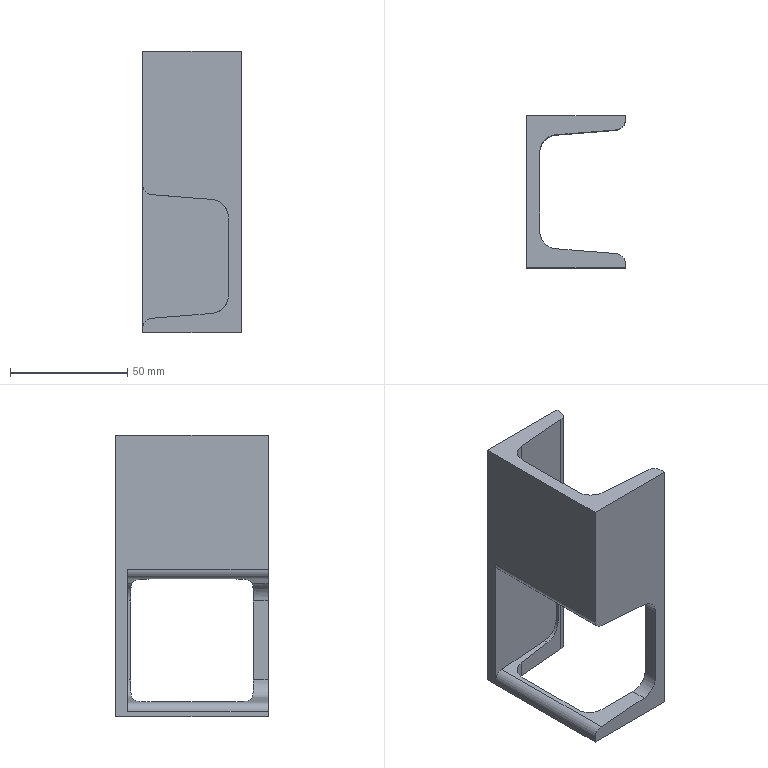Part | STEP file | DIN 1026-1 U 65 1785416005636 | 1 solid | 28 faces | box 42 x 65 x 120 mm | volume 74132 mm3 | plane 16 | cylinder 12 | commonest cylinder face diameters 15 x8 8 x4
STEP:
#1=CARTESIAN_POINT('',(29.598,-25.688,56.812));
#2=VERTEX_POINT('',#1);
#3=CARTESIAN_POINT('',(12.402,-24.312,58.188));
#4=VERTEX_POINT('',#3);
#5=CARTESIAN_POINT('',(10.69,-24.175,58.325));
#6=DIRECTION('',(-0.9937,0.07949,0.07949));
#7=VECTOR('',#6,10.);
#8=LINE('',#5,#7);
#9=EDGE_CURVE('',#2,#4,#8,.T.);
#10=ORIENTED_EDGE('',*,*,#9,.F.);
#11=CARTESIAN_POINT('',(29.598,-32.5,56.812));
#12=VERTEX_POINT('',#11);
#13=CARTESIAN_POINT('',(29.598,-32.5,56.812));
#14=DIRECTION('',(0.,1.,0.));
#15=VECTOR('',#14,10.);
#16=LINE('',#13,#15);
#17=EDGE_CURVE('',#12,#2,#16,.T.);
#18=ORIENTED_EDGE('',*,*,#17,.F.);
#19=CARTESIAN_POINT('',(3.681,-32.5,58.886));
#20=VERTEX_POINT('',#19);
#21=CARTESIAN_POINT('',(25.059,-32.5,57.175));
#22=DIRECTION('',(0.9968,0.,-0.07975));
#23=VECTOR('',#22,10.);
#24=LINE('',#21,#23);
#25=EDGE_CURVE('',#20,#12,#24,.T.);
#26=ORIENTED_EDGE('',*,*,#25,.F.);
#27=CARTESIAN_POINT('',(3.681,27.5,58.886));
#28=VERTEX_POINT('',#27);
#29=CARTESIAN_POINT('',(3.681,-32.5,58.886));
#30=DIRECTION('',(0.,1.,0.));
#31=VECTOR('',#30,10.);
#32=LINE('',#29,#31);
#33=EDGE_CURVE('',#20,#28,#32,.T.);
#34=ORIENTED_EDGE('',*,*,#33,.T.);
#35=CARTESIAN_POINT('',(29.598,27.5,56.812));
#36=VERTEX_POINT('',#35);
#37=CARTESIAN_POINT('',(29.598,27.5,56.812));
#38=DIRECTION('',(0.9968,0.,-0.07975));
#39=VECTOR('',#38,10.);
#40=LINE('',#37,#39);
#41=EDGE_CURVE('',#28,#36,#40,.T.);
#42=ORIENTED_EDGE('',*,*,#41,.T.);
#43=CARTESIAN_POINT('',(29.598,25.688,56.812));
#44=VERTEX_POINT('',#43);
#45=CARTESIAN_POINT('',(29.598,-32.5,56.812));
#46=DIRECTION('',(0.,1.,0.));
#47=VECTOR('',#46,10.);
#48=LINE('',#45,#47);
#49=EDGE_CURVE('',#44,#36,#48,.T.);
#50=ORIENTED_EDGE('',*,*,#49,.F.);
#51=CARTESIAN_POINT('',(12.402,24.312,58.188));
#52=VERTEX_POINT('',#51);
#53=CARTESIAN_POINT('',(21.,25.,57.5));
#54=DIRECTION('',(0.9937,0.07949,-0.07949));
#55=VECTOR('',#54,10.);
#56=LINE('',#53,#55);
#57=EDGE_CURVE('',#52,#44,#56,.T.);
#58=ORIENTED_EDGE('',*,*,#57,.F.);
#59=CARTESIAN_POINT('',(5.5,16.836,58.74));
#60=VERTEX_POINT('',#59);
#61=CARTESIAN_POINT('',(13.,16.836,58.14));
#62=DIRECTION('',(-0.07975,0.,-0.9968));
#63=DIRECTION('',(-0.9968,0.,0.07975));
#64=AXIS2_PLACEMENT_3D('',#61,#62,#63);
#65=ELLIPSE('',#64,7.524,7.5);
#66=EDGE_CURVE('',#60,#52,#65,.T.);
#67=ORIENTED_EDGE('',*,*,#66,.F.);
#68=CARTESIAN_POINT('',(5.5,-16.836,58.74));
#69=VERTEX_POINT('',#68);
#70=CARTESIAN_POINT('',(5.5,-16.25,58.74));
#71=DIRECTION('',(0.,1.,0.));
#72=VECTOR('',#71,10.);
#73=LINE('',#70,#72);
#74=EDGE_CURVE('',#69,#60,#73,.T.);
#75=ORIENTED_EDGE('',*,*,#74,.F.);
#76=CARTESIAN_POINT('',(13.,-16.836,58.14));
#77=DIRECTION('',(-0.07975,0.,-0.9968));
#78=DIRECTION('',(-0.9968,0.,0.07975));
#79=AXIS2_PLACEMENT_3D('',#76,#77,#78);
#80=ELLIPSE('',#79,7.524,7.5);
#81=EDGE_CURVE('',#4,#69,#80,.T.);
#82=ORIENTED_EDGE('',*,*,#81,.F.);
#83=EDGE_LOOP('',(#10,#18,#26,#34,#42,#50,#58,#67,#75,#82));
#84=FACE_OUTER_BOUND('',#83,.T.);
#85=CARTESIAN_POINT('',(3.681,-32.5,58.886));
#86=DIRECTION('',(0.07975,0.,0.9968));
#87=DIRECTION('',(0.9968,0.,-0.07975));
#88=AXIS2_PLACEMENT_3D('',#85,#86,#87);
#89=PLANE('',#88);
#90=ADVANCED_FACE('',(#84),#89,.F.);
#91=CARTESIAN_POINT('',(36.5,26.24,49.336));
#92=VERTEX_POINT('',#91);
#93=CARTESIAN_POINT('',(29.,25.64,49.336));
#94=DIRECTION('',(-0.07975,0.9968,0.));
#95=DIRECTION('',(0.9968,0.07975,0.));
#96=AXIS2_PLACEMENT_3D('',#93,#94,#95);
#97=ELLIPSE('',#96,7.524,7.5);
#98=EDGE_CURVE('',#44,#92,#97,.T.);
#99=ORIENTED_EDGE('',*,*,#98,.F.);
#100=ORIENTED_EDGE('',*,*,#49,.T.);
#101=CARTESIAN_POINT('',(36.5,27.5,49.336));
#102=VERTEX_POINT('',#101);
#103=CARTESIAN_POINT('',(29.,27.5,49.336));
#104=DIRECTION('',(0.,1.,0.));
#105=DIRECTION('',(1.,0.,0.));
#106=AXIS2_PLACEMENT_3D('',#103,#104,#105);
#107=CIRCLE('',#106,7.5);
#108=EDGE_CURVE('',#36,#102,#107,.T.);
#109=ORIENTED_EDGE('',*,*,#108,.T.);
#110=CARTESIAN_POINT('',(36.5,-32.5,49.336));
#111=DIRECTION('',(0.,1.,0.));
#112=VECTOR('',#111,10.);
#113=LINE('',#110,#112);
#114=EDGE_CURVE('',#92,#102,#113,.T.);
#115=ORIENTED_EDGE('',*,*,#114,.F.);
#116=EDGE_LOOP('',(#99,#100,#109,#115));
#117=FACE_OUTER_BOUND('',#116,.T.);
#118=CARTESIAN_POINT('',(29.,-32.5,49.336));
#119=DIRECTION('',(0.,1.,0.));
#120=DIRECTION('',(1.,0.,0.));
#121=AXIS2_PLACEMENT_3D('',#118,#119,#120);
#122=CYLINDRICAL_SURFACE('',#121,7.5);
#123=ADVANCED_FACE('',(#117),#122,.F.);
#124=CARTESIAN_POINT('',(36.5,26.24,15.664));
#125=VERTEX_POINT('',#124);
#126=CARTESIAN_POINT('',(36.5,26.24,24.668));
#127=DIRECTION('',(0.,0.,-1.));
#128=VECTOR('',#127,10.);
#129=LINE('',#126,#128);
#130=EDGE_CURVE('',#92,#125,#129,.T.);
#131=ORIENTED_EDGE('',*,*,#130,.F.);
#132=ORIENTED_EDGE('',*,*,#114,.T.);
#133=CARTESIAN_POINT('',(36.5,27.5,15.664));
#134=VERTEX_POINT('',#133);
#135=CARTESIAN_POINT('',(36.5,27.5,15.664));
#136=DIRECTION('',(0.,0.,-1.));
#137=VECTOR('',#136,10.);
#138=LINE('',#135,#137);
#139=EDGE_CURVE('',#102,#134,#138,.T.);
#140=ORIENTED_EDGE('',*,*,#139,.T.);
#141=CARTESIAN_POINT('',(36.5,-32.5,15.664));
#142=DIRECTION('',(0.,1.,0.));
#143=VECTOR('',#142,10.);
#144=LINE('',#141,#143);
#145=EDGE_CURVE('',#125,#134,#144,.T.);
#146=ORIENTED_EDGE('',*,*,#145,.F.);
#147=EDGE_LOOP('',(#131,#132,#140,#146));
#148=FACE_OUTER_BOUND('',#147,.T.);
#149=CARTESIAN_POINT('',(36.5,-32.5,49.336));
#150=DIRECTION('',(1.,0.,0.));
#151=DIRECTION('',(0.,0.,-1.));
#152=AXIS2_PLACEMENT_3D('',#149,#150,#151);
#153=PLANE('',#152);
#154=ADVANCED_FACE('',(#148),#153,.F.);
#155=CARTESIAN_POINT('',(29.598,25.688,8.188));
#156=VERTEX_POINT('',#155);
#157=CARTESIAN_POINT('',(29.,25.64,15.664));
#158=DIRECTION('',(-0.07975,0.9968,0.));
#159=DIRECTION('',(0.9968,0.07975,0.));
#160=AXIS2_PLACEMENT_3D('',#157,#158,#159);
#161=ELLIPSE('',#160,7.524,7.5);
#162=EDGE_CURVE('',#125,#156,#161,.T.);
#163=ORIENTED_EDGE('',*,*,#162,.F.);
#164=ORIENTED_EDGE('',*,*,#145,.T.);
#165=CARTESIAN_POINT('',(29.598,27.5,8.188));
#166=VERTEX_POINT('',#165);
#167=CARTESIAN_POINT('',(29.,27.5,15.664));
#168=DIRECTION('',(0.,1.,0.));
#169=DIRECTION('',(0.07975,0.,-0.9968));
#170=AXIS2_PLACEMENT_3D('',#167,#168,#169);
#171=CIRCLE('',#170,7.5);
#172=EDGE_CURVE('',#134,#166,#171,.T.);
#173=ORIENTED_EDGE('',*,*,#172,.T.);
#174=CARTESIAN_POINT('',(29.598,-32.5,8.188));
#175=DIRECTION('',(0.,1.,0.));
#176=VECTOR('',#175,10.);
#177=LINE('',#174,#176);
#178=EDGE_CURVE('',#156,#166,#177,.T.);
#179=ORIENTED_EDGE('',*,*,#178,.F.);
#180=EDGE_LOOP('',(#163,#164,#173,#179));
#181=FACE_OUTER_BOUND('',#180,.T.);
#182=CARTESIAN_POINT('',(29.,-32.5,15.664));
#183=DIRECTION('',(0.,1.,0.));
#184=DIRECTION('',(0.07975,0.,-0.9968));
#185=AXIS2_PLACEMENT_3D('',#182,#183,#184);
#186=CYLINDRICAL_SURFACE('',#185,7.5);
#187=ADVANCED_FACE('',(#181),#186,.F.);
#188=CARTESIAN_POINT('',(36.5,-26.24,15.664));
#189=VERTEX_POINT('',#188);
#190=CARTESIAN_POINT('',(36.5,-26.24,49.336));
#191=VERTEX_POINT('',#190);
#192=CARTESIAN_POINT('',(36.5,-26.24,24.668));
#193=DIRECTION('',(0.,0.,1.));
#194=VECTOR('',#193,10.);
#195=LINE('',#192,#194);
#196=EDGE_CURVE('',#189,#191,#195,.T.);
#197=ORIENTED_EDGE('',*,*,#196,.F.);
#198=CARTESIAN_POINT('',(36.5,-32.5,15.664));
#199=VERTEX_POINT('',#198);
#200=CARTESIAN_POINT('',(36.5,-32.5,15.664));
#201=DIRECTION('',(0.,1.,0.));
#202=VECTOR('',#201,10.);
#203=LINE('',#200,#202);
#204=EDGE_CURVE('',#199,#189,#203,.T.);
#205=ORIENTED_EDGE('',*,*,#204,.F.);
#206=CARTESIAN_POINT('',(36.5,-32.5,49.336));
#207=VERTEX_POINT('',#206);
#208=CARTESIAN_POINT('',(36.5,-32.5,24.668));
#209=DIRECTION('',(0.,0.,-1.));
#210=VECTOR('',#209,10.);
#211=LINE('',#208,#210);
#212=EDGE_CURVE('',#207,#199,#211,.T.);
#213=ORIENTED_EDGE('',*,*,#212,.F.);
#214=CARTESIAN_POINT('',(36.5,-32.5,49.336));
#215=DIRECTION('',(0.,1.,0.));
#216=VECTOR('',#215,10.);
#217=LINE('',#214,#216);
#218=EDGE_CURVE('',#207,#191,#217,.T.);
#219=ORIENTED_EDGE('',*,*,#218,.T.);
#220=EDGE_LOOP('',(#197,#205,#213,#219));
#221=FACE_OUTER_BOUND('',#220,.T.);
#222=CARTESIAN_POINT('',(36.5,-32.5,49.336));
#223=DIRECTION('',(1.,0.,0.));
#224=DIRECTION('',(0.,0.,-1.));
#225=AXIS2_PLACEMENT_3D('',#222,#223,#224);
#226=PLANE('',#225);
#227=ADVANCED_FACE('',(#221),#226,.F.);
#228=CARTESIAN_POINT('',(29.,-25.64,49.336));
#229=DIRECTION('',(-0.07975,-0.9968,0.));
#230=DIRECTION('',(0.9968,-0.07975,0.));
#231=AXIS2_PLACEMENT_3D('',#228,#229,#230);
#232=ELLIPSE('',#231,7.524,7.5);
#233=EDGE_CURVE('',#191,#2,#232,.T.);
#234=ORIENTED_EDGE('',*,*,#233,.F.);
#235=ORIENTED_EDGE('',*,*,#218,.F.);
#236=CARTESIAN_POINT('',(29.,-32.5,49.336));
#237=DIRECTION('',(0.,1.,0.));
#238=DIRECTION('',(1.,0.,0.));
#239=AXIS2_PLACEMENT_3D('',#236,#237,#238);
#240=CIRCLE('',#239,7.5);
#241=EDGE_CURVE('',#12,#207,#240,.T.);
#242=ORIENTED_EDGE('',*,*,#241,.F.);
#243=ORIENTED_EDGE('',*,*,#17,.T.);
#244=EDGE_LOOP('',(#234,#235,#242,#243));
#245=FACE_OUTER_BOUND('',#244,.T.);
#246=CARTESIAN_POINT('',(29.,-32.5,49.336));
#247=DIRECTION('',(0.,1.,0.));
#248=DIRECTION('',(1.,0.,0.));
#249=AXIS2_PLACEMENT_3D('',#246,#247,#248);
#250=CYLINDRICAL_SURFACE('',#249,7.5);
#251=ADVANCED_FACE('',(#245),#250,.F.);
#252=CARTESIAN_POINT('',(0.,-32.5,62.873));
#253=VERTEX_POINT('',#252);
#254=CARTESIAN_POINT('',(4.,-32.5,62.873));
#255=DIRECTION('',(0.,-1.,0.));
#256=DIRECTION('',(1.,0.,0.));
#257=AXIS2_PLACEMENT_3D('',#254,#255,#256);
#258=CIRCLE('',#257,4.);
#259=EDGE_CURVE('',#253,#20,#258,.T.);
#260=ORIENTED_EDGE('',*,*,#259,.F.);
#261=CARTESIAN_POINT('',(0.,27.5,62.873));
#262=VERTEX_POINT('',#261);
#263=CARTESIAN_POINT('',(0.,-32.5,62.873));
#264=DIRECTION('',(0.,-1.,0.));
#265=VECTOR('',#264,10.);
#266=LINE('',#263,#265);
#267=EDGE_CURVE('',#262,#253,#266,.T.);
#268=ORIENTED_EDGE('',*,*,#267,.F.);
#269=CARTESIAN_POINT('',(4.,27.5,62.873));
#270=DIRECTION('',(0.,-1.,0.));
#271=DIRECTION('',(1.,0.,0.));
#272=AXIS2_PLACEMENT_3D('',#269,#270,#271);
#273=CIRCLE('',#272,4.);
#274=EDGE_CURVE('',#262,#28,#273,.T.);
#275=ORIENTED_EDGE('',*,*,#274,.T.);
#276=ORIENTED_EDGE('',*,*,#33,.F.);
#277=EDGE_LOOP('',(#260,#268,#275,#276));
#278=FACE_OUTER_BOUND('',#277,.T.);
#279=CARTESIAN_POINT('',(4.,-32.5,62.873));
#280=DIRECTION('',(0.,1.,0.));
#281=DIRECTION('',(1.,0.,0.));
#282=AXIS2_PLACEMENT_3D('',#279,#280,#281);
#283=CYLINDRICAL_SURFACE('',#282,4.);
#284=ADVANCED_FACE('',(#278),#283,.T.);
#285=CARTESIAN_POINT('',(3.681,-32.5,6.114));
#286=VERTEX_POINT('',#285);
#287=CARTESIAN_POINT('',(0.,-32.5,2.127));
#288=VERTEX_POINT('',#287);
#289=CARTESIAN_POINT('',(4.,-32.5,2.127));
#290=DIRECTION('',(0.,-1.,0.));
#291=DIRECTION('',(0.07975,0.,-0.9968));
#292=AXIS2_PLACEMENT_3D('',#289,#290,#291);
#293=CIRCLE('',#292,4.);
#294=EDGE_CURVE('',#286,#288,#293,.T.);
#295=ORIENTED_EDGE('',*,*,#294,.F.);
#296=CARTESIAN_POINT('',(3.681,27.5,6.114));
#297=VERTEX_POINT('',#296);
#298=CARTESIAN_POINT('',(3.681,-32.5,6.114));
#299=DIRECTION('',(0.,1.,0.));
#300=VECTOR('',#299,10.);
#301=LINE('',#298,#300);
#302=EDGE_CURVE('',#286,#297,#301,.T.);
#303=ORIENTED_EDGE('',*,*,#302,.T.);
#304=CARTESIAN_POINT('',(0.,27.5,2.127));
#305=VERTEX_POINT('',#304);
#306=CARTESIAN_POINT('',(4.,27.5,2.127));
#307=DIRECTION('',(0.,-1.,0.));
#308=DIRECTION('',(0.07975,0.,-0.9968));
#309=AXIS2_PLACEMENT_3D('',#306,#307,#308);
#310=CIRCLE('',#309,4.);
#311=EDGE_CURVE('',#297,#305,#310,.T.);
#312=ORIENTED_EDGE('',*,*,#311,.T.);
#313=CARTESIAN_POINT('',(0.,-32.5,2.127));
#314=DIRECTION('',(0.,-1.,0.));
#315=VECTOR('',#314,10.);
#316=LINE('',#313,#315);
#317=EDGE_CURVE('',#305,#288,#316,.T.);
#318=ORIENTED_EDGE('',*,*,#317,.T.);
#319=EDGE_LOOP('',(#295,#303,#312,#318));
#320=FACE_OUTER_BOUND('',#319,.T.);
#321=CARTESIAN_POINT('',(4.,-32.5,2.127));
#322=DIRECTION('',(0.,1.,0.));
#323=DIRECTION('',(0.07975,0.,-0.9968));
#324=AXIS2_PLACEMENT_3D('',#321,#322,#323);
#325=CYLINDRICAL_SURFACE('',#324,4.);
#326=ADVANCED_FACE('',(#320),#325,.T.);
#327=CARTESIAN_POINT('',(12.402,-24.312,6.812));
#328=VERTEX_POINT('',#327);
#329=CARTESIAN_POINT('',(29.598,-25.688,8.188));
#330=VERTEX_POINT('',#329);
#331=CARTESIAN_POINT('',(21.,-25.,7.5));
#332=DIRECTION('',(0.9937,-0.07949,0.07949));
#333=VECTOR('',#332,10.);
#334=LINE('',#331,#333);
#335=EDGE_CURVE('',#328,#330,#334,.T.);
#336=ORIENTED_EDGE('',*,*,#335,.F.);
#337=CARTESIAN_POINT('',(5.5,-16.836,6.26));
#338=VERTEX_POINT('',#337);
#339=CARTESIAN_POINT('',(13.,-16.836,6.86));
#340=DIRECTION('',(-0.07975,0.,0.9968));
#341=DIRECTION('',(-0.9968,0.,-0.07975));
#342=AXIS2_PLACEMENT_3D('',#339,#340,#341);
#343=ELLIPSE('',#342,7.524,7.5);
#344=EDGE_CURVE('',#338,#328,#343,.T.);
#345=ORIENTED_EDGE('',*,*,#344,.F.);
#346=CARTESIAN_POINT('',(5.5,16.836,6.26));
#347=VERTEX_POINT('',#346);
#348=CARTESIAN_POINT('',(5.5,-16.25,6.26));
#349=DIRECTION('',(0.,-1.,0.));
#350=VECTOR('',#349,10.);
#351=LINE('',#348,#350);
#352=EDGE_CURVE('',#347,#338,#351,.T.);
#353=ORIENTED_EDGE('',*,*,#352,.F.);
#354=CARTESIAN_POINT('',(12.402,24.312,6.812));
#355=VERTEX_POINT('',#354);
#356=CARTESIAN_POINT('',(13.,16.836,6.86));
#357=DIRECTION('',(-0.07975,0.,0.9968));
#358=DIRECTION('',(-0.9968,0.,-0.07975));
#359=AXIS2_PLACEMENT_3D('',#356,#357,#358);
#360=ELLIPSE('',#359,7.524,7.5);
#361=EDGE_CURVE('',#355,#347,#360,.T.);
#362=ORIENTED_EDGE('',*,*,#361,.F.);
#363=CARTESIAN_POINT('',(31.31,25.825,8.325));
#364=DIRECTION('',(-0.9937,-0.07949,-0.07949));
#365=VECTOR('',#364,10.);
#366=LINE('',#363,#365);
#367=EDGE_CURVE('',#156,#355,#366,.T.);
#368=ORIENTED_EDGE('',*,*,#367,.F.);
#369=ORIENTED_EDGE('',*,*,#178,.T.);
#370=CARTESIAN_POINT('',(3.681,27.5,6.114));
#371=DIRECTION('',(-0.9968,0.,-0.07975));
#372=VECTOR('',#371,10.);
#373=LINE('',#370,#372);
#374=EDGE_CURVE('',#166,#297,#373,.T.);
#375=ORIENTED_EDGE('',*,*,#374,.T.);
#376=ORIENTED_EDGE('',*,*,#302,.F.);
#377=CARTESIAN_POINT('',(29.598,-32.5,8.188));
#378=VERTEX_POINT('',#377);
#379=CARTESIAN_POINT('',(35.434,-32.5,8.655));
#380=DIRECTION('',(-0.9968,0.,-0.07975));
#381=VECTOR('',#380,10.);
#382=LINE('',#379,#381);
#383=EDGE_CURVE('',#378,#286,#382,.T.);
#384=ORIENTED_EDGE('',*,*,#383,.F.);
#385=CARTESIAN_POINT('',(29.598,-32.5,8.188));
#386=DIRECTION('',(0.,1.,0.));
#387=VECTOR('',#386,10.);
#388=LINE('',#385,#387);
#389=EDGE_CURVE('',#378,#330,#388,.T.);
#390=ORIENTED_EDGE('',*,*,#389,.T.);
#391=EDGE_LOOP('',(#336,#345,#353,#362,#368,#369,#375,#376,#384,#390));
#392=FACE_OUTER_BOUND('',#391,.T.);
#393=CARTESIAN_POINT('',(29.598,-32.5,8.188));
#394=DIRECTION('',(0.07975,0.,-0.9968));
#395=DIRECTION('',(-0.9968,0.,-0.07975));
#396=AXIS2_PLACEMENT_3D('',#393,#394,#395);
#397=PLANE('',#396);
#398=ADVANCED_FACE('',(#392),#397,.F.);
#399=CARTESIAN_POINT('',(29.,-25.64,15.664));
#400=DIRECTION('',(-0.07975,-0.9968,0.));
#401=DIRECTION('',(0.9968,-0.07975,0.));
#402=AXIS2_PLACEMENT_3D('',#399,#400,#401);
#403=ELLIPSE('',#402,7.524,7.5);
#404=EDGE_CURVE('',#330,#189,#403,.T.);
#405=ORIENTED_EDGE('',*,*,#404,.F.);
#406=ORIENTED_EDGE('',*,*,#389,.F.);
#407=CARTESIAN_POINT('',(29.,-32.5,15.664));
#408=DIRECTION('',(0.,1.,0.));
#409=DIRECTION('',(0.07975,0.,-0.9968));
#410=AXIS2_PLACEMENT_3D('',#407,#408,#409);
#411=CIRCLE('',#410,7.5);
#412=EDGE_CURVE('',#199,#378,#411,.T.);
#413=ORIENTED_EDGE('',*,*,#412,.F.);
#414=ORIENTED_EDGE('',*,*,#204,.T.);
#415=EDGE_LOOP('',(#405,#406,#413,#414));
#416=FACE_OUTER_BOUND('',#415,.T.);
#417=CARTESIAN_POINT('',(29.,-32.5,15.664));
#418=DIRECTION('',(0.,1.,0.));
#419=DIRECTION('',(0.07975,0.,-0.9968));
#420=AXIS2_PLACEMENT_3D('',#417,#418,#419);
#421=CYLINDRICAL_SURFACE('',#420,7.5);
#422=ADVANCED_FACE('',(#416),#421,.F.);
#423=ORIENTED_EDGE('',*,*,#172,.F.);
#424=ORIENTED_EDGE('',*,*,#139,.F.);
#425=ORIENTED_EDGE('',*,*,#108,.F.);
#426=ORIENTED_EDGE('',*,*,#41,.F.);
#427=ORIENTED_EDGE('',*,*,#274,.F.);
#428=CARTESIAN_POINT('',(0.,27.5,16.25));
#429=DIRECTION('',(0.,0.,1.));
#430=VECTOR('',#429,10.);
#431=LINE('',#428,#430);
#432=EDGE_CURVE('',#305,#262,#431,.T.);
#433=ORIENTED_EDGE('',*,*,#432,.F.);
#434=ORIENTED_EDGE('',*,*,#311,.F.);
#435=ORIENTED_EDGE('',*,*,#374,.F.);
#436=EDGE_LOOP('',(#423,#424,#425,#426,#427,#433,#434,#435));
#437=FACE_OUTER_BOUND('',#436,.T.);
#438=CARTESIAN_POINT('',(18.25,27.5,32.5));
#439=DIRECTION('',(0.,-1.,0.));
#440=DIRECTION('',(-1.,0.,0.));
#441=AXIS2_PLACEMENT_3D('',#438,#439,#440);
#442=PLANE('',#441);
#443=ADVANCED_FACE('',(#437),#442,.T.);
#444=ORIENTED_EDGE('',*,*,#317,.F.);
#445=ORIENTED_EDGE('',*,*,#432,.T.);
#446=ORIENTED_EDGE('',*,*,#267,.T.);
#447=CARTESIAN_POINT('',(0.,-32.5,120.));
#448=VERTEX_POINT('',#447);
#449=CARTESIAN_POINT('',(0.,-32.5,0.));
#450=DIRECTION('',(0.,0.,1.));
#451=VECTOR('',#450,10.);
#452=LINE('',#449,#451);
#453=EDGE_CURVE('',#253,#448,#452,.T.);
#454=ORIENTED_EDGE('',*,*,#453,.T.);
#455=CARTESIAN_POINT('',(0.,32.5,120.));
#456=VERTEX_POINT('',#455);
#457=CARTESIAN_POINT('',(0.,0.,120.));
#458=DIRECTION('',(0.,1.,0.));
#459=VECTOR('',#458,10.);
#460=LINE('',#457,#459);
#461=EDGE_CURVE('',#448,#456,#460,.T.);
#462=ORIENTED_EDGE('',*,*,#461,.T.);
#463=CARTESIAN_POINT('',(0.,32.5,0.));
#464=VERTEX_POINT('',#463);
#465=CARTESIAN_POINT('',(0.,32.5,0.));
#466=DIRECTION('',(0.,0.,1.));
#467=VECTOR('',#466,10.);
#468=LINE('',#465,#467);
#469=EDGE_CURVE('',#464,#456,#468,.T.);
#470=ORIENTED_EDGE('',*,*,#469,.F.);
#471=CARTESIAN_POINT('',(0.,-32.5,0.));
#472=VERTEX_POINT('',#471);
#473=CARTESIAN_POINT('',(0.,0.,0.));
#474=DIRECTION('',(0.,1.,0.));
#475=VECTOR('',#474,10.);
#476=LINE('',#473,#475);
#477=EDGE_CURVE('',#472,#464,#476,.T.);
#478=ORIENTED_EDGE('',*,*,#477,.F.);
#479=CARTESIAN_POINT('',(0.,-32.5,0.));
#480=DIRECTION('',(0.,0.,1.));
#481=VECTOR('',#480,10.);
#482=LINE('',#479,#481);
#483=EDGE_CURVE('',#472,#288,#482,.T.);
#484=ORIENTED_EDGE('',*,*,#483,.T.);
#485=EDGE_LOOP('',(#444,#445,#446,#454,#462,#470,#478,#484));
#486=FACE_OUTER_BOUND('',#485,.T.);
#487=CARTESIAN_POINT('',(0.,0.,0.));
#488=DIRECTION('',(-1.,0.,0.));
#489=DIRECTION('',(0.,0.,1.));
#490=AXIS2_PLACEMENT_3D('',#487,#488,#489);
#491=PLANE('',#490);
#492=ADVANCED_FACE('',(#486),#491,.T.);
#493=ORIENTED_EDGE('',*,*,#57,.T.);
#494=ORIENTED_EDGE('',*,*,#98,.T.);
#495=ORIENTED_EDGE('',*,*,#130,.T.);
#496=ORIENTED_EDGE('',*,*,#162,.T.);
#497=ORIENTED_EDGE('',*,*,#367,.T.);
#498=CARTESIAN_POINT('',(12.402,24.312,0.));
#499=VERTEX_POINT('',#498);
#500=CARTESIAN_POINT('',(12.402,24.312,0.));
#501=DIRECTION('',(0.,0.,1.));
#502=VECTOR('',#501,10.);
#503=LINE('',#500,#502);
#504=EDGE_CURVE('',#499,#355,#503,.T.);
#505=ORIENTED_EDGE('',*,*,#504,.F.);
#506=CARTESIAN_POINT('',(38.319,26.386,0.));
#507=VERTEX_POINT('',#506);
#508=CARTESIAN_POINT('',(28.666,25.613,0.));
#509=DIRECTION('',(-0.9968,-0.07975,0.));
#510=VECTOR('',#509,10.);
#511=LINE('',#508,#510);
#512=EDGE_CURVE('',#507,#499,#511,.T.);
#513=ORIENTED_EDGE('',*,*,#512,.F.);
#514=CARTESIAN_POINT('',(38.319,26.386,120.));
#515=VERTEX_POINT('',#514);
#516=CARTESIAN_POINT('',(38.319,26.386,0.));
#517=DIRECTION('',(0.,0.,1.));
#518=VECTOR('',#517,10.);
#519=LINE('',#516,#518);
#520=EDGE_CURVE('',#507,#515,#519,.T.);
#521=ORIENTED_EDGE('',*,*,#520,.T.);
#522=CARTESIAN_POINT('',(12.402,24.312,120.));
#523=VERTEX_POINT('',#522);
#524=CARTESIAN_POINT('',(28.666,25.613,120.));
#525=DIRECTION('',(-0.9968,-0.07975,0.));
#526=VECTOR('',#525,10.);
#527=LINE('',#524,#526);
#528=EDGE_CURVE('',#515,#523,#527,.T.);
#529=ORIENTED_EDGE('',*,*,#528,.T.);
#530=CARTESIAN_POINT('',(12.402,24.312,0.));
#531=DIRECTION('',(0.,0.,1.));
#532=VECTOR('',#531,10.);
#533=LINE('',#530,#532);
#534=EDGE_CURVE('',#52,#523,#533,.T.);
#535=ORIENTED_EDGE('',*,*,#534,.F.);
#536=EDGE_LOOP('',(#493,#494,#495,#496,#497,#505,#513,#521,#529,#535));
#537=FACE_OUTER_BOUND('',#536,.T.);
#538=CARTESIAN_POINT('',(38.319,26.386,0.));
#539=DIRECTION('',(0.07975,-0.9968,0.));
#540=DIRECTION('',(0.,0.,-1.));
#541=AXIS2_PLACEMENT_3D('',#538,#539,#540);
#542=PLANE('',#541);
#543=ADVANCED_FACE('',(#537),#542,.T.);
#544=ORIENTED_EDGE('',*,*,#344,.T.);
#545=CARTESIAN_POINT('',(12.402,-24.312,0.));
#546=VERTEX_POINT('',#545);
#547=CARTESIAN_POINT('',(12.402,-24.312,0.));
#548=DIRECTION('',(0.,0.,1.));
#549=VECTOR('',#548,10.);
#550=LINE('',#547,#549);
#551=EDGE_CURVE('',#546,#328,#550,.T.);
#552=ORIENTED_EDGE('',*,*,#551,.F.);
#553=CARTESIAN_POINT('',(5.5,-16.836,0.));
#554=VERTEX_POINT('',#553);
#555=CARTESIAN_POINT('',(13.,-16.836,0.));
#556=DIRECTION('',(0.,0.,1.));
#557=DIRECTION('',(-1.,0.,0.));
#558=AXIS2_PLACEMENT_3D('',#555,#556,#557);
#559=CIRCLE('',#558,7.5);
#560=EDGE_CURVE('',#554,#546,#559,.T.);
#561=ORIENTED_EDGE('',*,*,#560,.F.);
#562=CARTESIAN_POINT('',(5.5,-16.836,0.));
#563=DIRECTION('',(0.,0.,1.));
#564=VECTOR('',#563,10.);
#565=LINE('',#562,#564);
#566=EDGE_CURVE('',#554,#338,#565,.T.);
#567=ORIENTED_EDGE('',*,*,#566,.T.);
#568=EDGE_LOOP('',(#544,#552,#561,#567));
#569=FACE_OUTER_BOUND('',#568,.T.);
#570=CARTESIAN_POINT('',(13.,-16.836,0.));
#571=DIRECTION('',(0.,0.,1.));
#572=DIRECTION('',(-1.,0.,0.));
#573=AXIS2_PLACEMENT_3D('',#570,#571,#572);
#574=CYLINDRICAL_SURFACE('',#573,7.5);
#575=ADVANCED_FACE('',(#569),#574,.F.);
#576=ORIENTED_EDGE('',*,*,#81,.T.);
#577=CARTESIAN_POINT('',(5.5,-16.836,120.));
#578=VERTEX_POINT('',#577);
#579=CARTESIAN_POINT('',(5.5,-16.836,0.));
#580=DIRECTION('',(0.,0.,1.));
#581=VECTOR('',#580,10.);
#582=LINE('',#579,#581);
#583=EDGE_CURVE('',#69,#578,#582,.T.);
#584=ORIENTED_EDGE('',*,*,#583,.T.);
#585=CARTESIAN_POINT('',(12.402,-24.312,120.));
#586=VERTEX_POINT('',#585);
#587=CARTESIAN_POINT('',(13.,-16.836,120.));
#588=DIRECTION('',(0.,0.,1.));
#589=DIRECTION('',(-1.,0.,0.));
#590=AXIS2_PLACEMENT_3D('',#587,#588,#589);
#591=CIRCLE('',#590,7.5);
#592=EDGE_CURVE('',#578,#586,#591,.T.);
#593=ORIENTED_EDGE('',*,*,#592,.T.);
#594=CARTESIAN_POINT('',(12.402,-24.312,0.));
#595=DIRECTION('',(0.,0.,1.));
#596=VECTOR('',#595,10.);
#597=LINE('',#594,#596);
#598=EDGE_CURVE('',#4,#586,#597,.T.);
#599=ORIENTED_EDGE('',*,*,#598,.F.);
#600=EDGE_LOOP('',(#576,#584,#593,#599));
#601=FACE_OUTER_BOUND('',#600,.T.);
#602=CARTESIAN_POINT('',(13.,-16.836,0.));
#603=DIRECTION('',(0.,0.,1.));
#604=DIRECTION('',(-1.,0.,0.));
#605=AXIS2_PLACEMENT_3D('',#602,#603,#604);
#606=CYLINDRICAL_SURFACE('',#605,7.5);
#607=ADVANCED_FACE('',(#601),#606,.F.);
#608=ORIENTED_EDGE('',*,*,#352,.T.);
#609=ORIENTED_EDGE('',*,*,#566,.F.);
#610=CARTESIAN_POINT('',(5.5,16.836,0.));
#611=VERTEX_POINT('',#610);
#612=CARTESIAN_POINT('',(5.5,0.,0.));
#613=DIRECTION('',(0.,-1.,0.));
#614=VECTOR('',#613,10.);
#615=LINE('',#612,#614);
#616=EDGE_CURVE('',#611,#554,#615,.T.);
#617=ORIENTED_EDGE('',*,*,#616,.F.);
#618=CARTESIAN_POINT('',(5.5,16.836,0.));
#619=DIRECTION('',(0.,0.,1.));
#620=VECTOR('',#619,10.);
#621=LINE('',#618,#620);
#622=EDGE_CURVE('',#611,#347,#621,.T.);
#623=ORIENTED_EDGE('',*,*,#622,.T.);
#624=EDGE_LOOP('',(#608,#609,#617,#623));
#625=FACE_OUTER_BOUND('',#624,.T.);
#626=CARTESIAN_POINT('',(5.5,0.,0.));
#627=DIRECTION('',(1.,0.,0.));
#628=DIRECTION('',(0.,0.,-1.));
#629=AXIS2_PLACEMENT_3D('',#626,#627,#628);
#630=PLANE('',#629);
#631=ADVANCED_FACE('',(#625),#630,.T.);
#632=ORIENTED_EDGE('',*,*,#74,.T.);
#633=CARTESIAN_POINT('',(5.5,16.836,120.));
#634=VERTEX_POINT('',#633);
#635=CARTESIAN_POINT('',(5.5,16.836,0.));
#636=DIRECTION('',(0.,0.,1.));
#637=VECTOR('',#636,10.);
#638=LINE('',#635,#637);
#639=EDGE_CURVE('',#60,#634,#638,.T.);
#640=ORIENTED_EDGE('',*,*,#639,.T.);
#641=CARTESIAN_POINT('',(5.5,0.,120.));
#642=DIRECTION('',(0.,-1.,0.));
#643=VECTOR('',#642,10.);
#644=LINE('',#641,#643);
#645=EDGE_CURVE('',#634,#578,#644,.T.);
#646=ORIENTED_EDGE('',*,*,#645,.T.);
#647=ORIENTED_EDGE('',*,*,#583,.F.);
#648=EDGE_LOOP('',(#632,#640,#646,#647));
#649=FACE_OUTER_BOUND('',#648,.T.);
#650=CARTESIAN_POINT('',(5.5,0.,0.));
#651=DIRECTION('',(1.,0.,0.));
#652=DIRECTION('',(0.,0.,-1.));
#653=AXIS2_PLACEMENT_3D('',#650,#651,#652);
#654=PLANE('',#653);
#655=ADVANCED_FACE('',(#649),#654,.T.);
#656=ORIENTED_EDGE('',*,*,#361,.T.);
#657=ORIENTED_EDGE('',*,*,#622,.F.);
#658=CARTESIAN_POINT('',(13.,16.836,0.));
#659=DIRECTION('',(0.,0.,1.));
#660=DIRECTION('',(-0.07975,0.9968,0.));
#661=AXIS2_PLACEMENT_3D('',#658,#659,#660);
#662=CIRCLE('',#661,7.5);
#663=EDGE_CURVE('',#499,#611,#662,.T.);
#664=ORIENTED_EDGE('',*,*,#663,.F.);
#665=ORIENTED_EDGE('',*,*,#504,.T.);
#666=EDGE_LOOP('',(#656,#657,#664,#665));
#667=FACE_OUTER_BOUND('',#666,.T.);
#668=CARTESIAN_POINT('',(13.,16.836,0.));
#669=DIRECTION('',(0.,0.,1.));
#670=DIRECTION('',(-0.07975,0.9968,0.));
#671=AXIS2_PLACEMENT_3D('',#668,#669,#670);
#672=CYLINDRICAL_SURFACE('',#671,7.5);
#673=ADVANCED_FACE('',(#667),#672,.F.);
#674=ORIENTED_EDGE('',*,*,#66,.T.);
#675=ORIENTED_EDGE('',*,*,#534,.T.);
#676=CARTESIAN_POINT('',(13.,16.836,120.));
#677=DIRECTION('',(0.,0.,1.));
#678=DIRECTION('',(-0.07975,0.9968,0.));
#679=AXIS2_PLACEMENT_3D('',#676,#677,#678);
#680=CIRCLE('',#679,7.5);
#681=EDGE_CURVE('',#523,#634,#680,.T.);
#682=ORIENTED_EDGE('',*,*,#681,.T.);
#683=ORIENTED_EDGE('',*,*,#639,.F.);
#684=EDGE_LOOP('',(#674,#675,#682,#683));
#685=FACE_OUTER_BOUND('',#684,.T.);
#686=CARTESIAN_POINT('',(13.,16.836,0.));
#687=DIRECTION('',(0.,0.,1.));
#688=DIRECTION('',(-0.07975,0.9968,0.));
#689=AXIS2_PLACEMENT_3D('',#686,#687,#688);
#690=CYLINDRICAL_SURFACE('',#689,7.5);
#691=ADVANCED_FACE('',(#685),#690,.F.);
#692=ORIENTED_EDGE('',*,*,#9,.T.);
#693=ORIENTED_EDGE('',*,*,#598,.T.);
#694=CARTESIAN_POINT('',(38.319,-26.386,120.));
#695=VERTEX_POINT('',#694);
#696=CARTESIAN_POINT('',(15.707,-24.577,120.));
#697=DIRECTION('',(0.9968,-0.07975,0.));
#698=VECTOR('',#697,10.);
#699=LINE('',#696,#698);
#700=EDGE_CURVE('',#586,#695,#699,.T.);
#701=ORIENTED_EDGE('',*,*,#700,.T.);
#702=CARTESIAN_POINT('',(38.319,-26.386,0.));
#703=VERTEX_POINT('',#702);
#704=CARTESIAN_POINT('',(38.319,-26.386,0.));
#705=DIRECTION('',(0.,0.,1.));
#706=VECTOR('',#705,10.);
#707=LINE('',#704,#706);
#708=EDGE_CURVE('',#703,#695,#707,.T.);
#709=ORIENTED_EDGE('',*,*,#708,.F.);
#710=CARTESIAN_POINT('',(15.707,-24.577,0.));
#711=DIRECTION('',(0.9968,-0.07975,0.));
#712=VECTOR('',#711,10.);
#713=LINE('',#710,#712);
#714=EDGE_CURVE('',#546,#703,#713,.T.);
#715=ORIENTED_EDGE('',*,*,#714,.F.);
#716=ORIENTED_EDGE('',*,*,#551,.T.);
#717=ORIENTED_EDGE('',*,*,#335,.T.);
#718=ORIENTED_EDGE('',*,*,#404,.T.);
#719=ORIENTED_EDGE('',*,*,#196,.T.);
#720=ORIENTED_EDGE('',*,*,#233,.T.);
#721=EDGE_LOOP('',(#692,#693,#701,#709,#715,#716,#717,#718,#719,#720));
#722=FACE_OUTER_BOUND('',#721,.T.);
#723=CARTESIAN_POINT('',(12.402,-24.312,0.));
#724=DIRECTION('',(0.07975,0.9968,0.));
#725=DIRECTION('',(0.,0.,1.));
#726=AXIS2_PLACEMENT_3D('',#723,#724,#725);
#727=PLANE('',#726);
#728=ADVANCED_FACE('',(#722),#727,.T.);
#729=CARTESIAN_POINT('',(42.,-30.373,120.));
#730=VERTEX_POINT('',#729);
#731=CARTESIAN_POINT('',(38.,-30.373,120.));
#732=DIRECTION('',(0.,0.,-1.));
#733=DIRECTION('',(-1.,0.,0.));
#734=AXIS2_PLACEMENT_3D('',#731,#732,#733);
#735=CIRCLE('',#734,4.);
#736=EDGE_CURVE('',#695,#730,#735,.T.);
#737=ORIENTED_EDGE('',*,*,#736,.T.);
#738=CARTESIAN_POINT('',(42.,-30.373,0.));
#739=VERTEX_POINT('',#738);
#740=CARTESIAN_POINT('',(42.,-30.373,0.));
#741=DIRECTION('',(0.,0.,1.));
#742=VECTOR('',#741,10.);
#743=LINE('',#740,#742);
#744=EDGE_CURVE('',#739,#730,#743,.T.);
#745=ORIENTED_EDGE('',*,*,#744,.F.);
#746=CARTESIAN_POINT('',(38.,-30.373,0.));
#747=DIRECTION('',(0.,0.,-1.));
#748=DIRECTION('',(-1.,0.,0.));
#749=AXIS2_PLACEMENT_3D('',#746,#747,#748);
#750=CIRCLE('',#749,4.);
#751=EDGE_CURVE('',#703,#739,#750,.T.);
#752=ORIENTED_EDGE('',*,*,#751,.F.);
#753=ORIENTED_EDGE('',*,*,#708,.T.);
#754=EDGE_LOOP('',(#737,#745,#752,#753));
#755=FACE_OUTER_BOUND('',#754,.T.);
#756=CARTESIAN_POINT('',(38.,-30.373,0.));
#757=DIRECTION('',(0.,0.,1.));
#758=DIRECTION('',(-1.,0.,0.));
#759=AXIS2_PLACEMENT_3D('',#756,#757,#758);
#760=CYLINDRICAL_SURFACE('',#759,4.);
#761=ADVANCED_FACE('',(#755),#760,.T.);
#762=CARTESIAN_POINT('',(42.,-32.5,120.));
#763=VERTEX_POINT('',#762);
#764=CARTESIAN_POINT('',(42.,-15.186,120.));
#765=DIRECTION('',(0.,-1.,0.));
#766=VECTOR('',#765,10.);
#767=LINE('',#764,#766);
#768=EDGE_CURVE('',#730,#763,#767,.T.);
#769=ORIENTED_EDGE('',*,*,#768,.T.);
#770=CARTESIAN_POINT('',(42.,-32.5,0.));
#771=VERTEX_POINT('',#770);
#772=CARTESIAN_POINT('',(42.,-32.5,0.));
#773=DIRECTION('',(0.,0.,1.));
#774=VECTOR('',#773,10.);
#775=LINE('',#772,#774);
#776=EDGE_CURVE('',#771,#763,#775,.T.);
#777=ORIENTED_EDGE('',*,*,#776,.F.);
#778=CARTESIAN_POINT('',(42.,-15.186,0.));
#779=DIRECTION('',(0.,-1.,0.));
#780=VECTOR('',#779,10.);
#781=LINE('',#778,#780);
#782=EDGE_CURVE('',#739,#771,#781,.T.);
#783=ORIENTED_EDGE('',*,*,#782,.F.);
#784=ORIENTED_EDGE('',*,*,#744,.T.);
#785=EDGE_LOOP('',(#769,#777,#783,#784));
#786=FACE_OUTER_BOUND('',#785,.T.);
#787=CARTESIAN_POINT('',(42.,-30.373,0.));
#788=DIRECTION('',(1.,0.,0.));
#789=DIRECTION('',(0.,0.,-1.));
#790=AXIS2_PLACEMENT_3D('',#787,#788,#789);
#791=PLANE('',#790);
#792=ADVANCED_FACE('',(#786),#791,.T.);
#793=ORIENTED_EDGE('',*,*,#294,.T.);
#794=ORIENTED_EDGE('',*,*,#483,.F.);
#795=CARTESIAN_POINT('',(31.5,-32.5,0.));
#796=DIRECTION('',(-1.,0.,0.));
#797=VECTOR('',#796,10.);
#798=LINE('',#795,#797);
#799=EDGE_CURVE('',#771,#472,#798,.T.);
#800=ORIENTED_EDGE('',*,*,#799,.F.);
#801=ORIENTED_EDGE('',*,*,#776,.T.);
#802=CARTESIAN_POINT('',(31.5,-32.5,120.));
#803=DIRECTION('',(-1.,0.,0.));
#804=VECTOR('',#803,10.);
#805=LINE('',#802,#804);
#806=EDGE_CURVE('',#763,#448,#805,.T.);
#807=ORIENTED_EDGE('',*,*,#806,.T.);
#808=ORIENTED_EDGE('',*,*,#453,.F.);
#809=ORIENTED_EDGE('',*,*,#259,.T.);
#810=ORIENTED_EDGE('',*,*,#25,.T.);
#811=ORIENTED_EDGE('',*,*,#241,.T.);
#812=ORIENTED_EDGE('',*,*,#212,.T.);
#813=ORIENTED_EDGE('',*,*,#412,.T.);
#814=ORIENTED_EDGE('',*,*,#383,.T.);
#815=EDGE_LOOP('',(#793,#794,#800,#801,#807,#808,#809,#810,#811,#812,#813,#814));
#816=FACE_OUTER_BOUND('',#815,.T.);
#817=CARTESIAN_POINT('',(42.,-32.5,0.));
#818=DIRECTION('',(0.,-1.,0.));
#819=DIRECTION('',(0.,0.,-1.));
#820=AXIS2_PLACEMENT_3D('',#817,#818,#819);
#821=PLANE('',#820);
#822=ADVANCED_FACE('',(#816),#821,.T.);
#823=CARTESIAN_POINT('',(42.,32.5,120.));
#824=VERTEX_POINT('',#823);
#825=CARTESIAN_POINT('',(10.5,32.5,120.));
#826=DIRECTION('',(1.,0.,0.));
#827=VECTOR('',#826,10.);
#828=LINE('',#825,#827);
#829=EDGE_CURVE('',#456,#824,#828,.T.);
#830=ORIENTED_EDGE('',*,*,#829,.T.);
#831=CARTESIAN_POINT('',(42.,32.5,0.));
#832=VERTEX_POINT('',#831);
#833=CARTESIAN_POINT('',(42.,32.5,0.));
#834=DIRECTION('',(0.,0.,1.));
#835=VECTOR('',#834,10.);
#836=LINE('',#833,#835);
#837=EDGE_CURVE('',#832,#824,#836,.T.);
#838=ORIENTED_EDGE('',*,*,#837,.F.);
#839=CARTESIAN_POINT('',(10.5,32.5,0.));
#840=DIRECTION('',(1.,0.,0.));
#841=VECTOR('',#840,10.);
#842=LINE('',#839,#841);
#843=EDGE_CURVE('',#464,#832,#842,.T.);
#844=ORIENTED_EDGE('',*,*,#843,.F.);
#845=ORIENTED_EDGE('',*,*,#469,.T.);
#846=EDGE_LOOP('',(#830,#838,#844,#845));
#847=FACE_OUTER_BOUND('',#846,.T.);
#848=CARTESIAN_POINT('',(0.,32.5,0.));
#849=DIRECTION('',(0.,1.,0.));
#850=DIRECTION('',(0.,0.,1.));
#851=AXIS2_PLACEMENT_3D('',#848,#849,#850);
#852=PLANE('',#851);
#853=ADVANCED_FACE('',(#847),#852,.T.);
#854=CARTESIAN_POINT('',(42.,30.373,120.));
#855=VERTEX_POINT('',#854);
#856=CARTESIAN_POINT('',(42.,16.25,120.));
#857=DIRECTION('',(0.,-1.,0.));
#858=VECTOR('',#857,10.);
#859=LINE('',#856,#858);
#860=EDGE_CURVE('',#824,#855,#859,.T.);
#861=ORIENTED_EDGE('',*,*,#860,.T.);
#862=CARTESIAN_POINT('',(42.,30.373,0.));
#863=VERTEX_POINT('',#862);
#864=CARTESIAN_POINT('',(42.,30.373,0.));
#865=DIRECTION('',(0.,0.,1.));
#866=VECTOR('',#865,10.);
#867=LINE('',#864,#866);
#868=EDGE_CURVE('',#863,#855,#867,.T.);
#869=ORIENTED_EDGE('',*,*,#868,.F.);
#870=CARTESIAN_POINT('',(42.,16.25,0.));
#871=DIRECTION('',(0.,-1.,0.));
#872=VECTOR('',#871,10.);
#873=LINE('',#870,#872);
#874=EDGE_CURVE('',#832,#863,#873,.T.);
#875=ORIENTED_EDGE('',*,*,#874,.F.);
#876=ORIENTED_EDGE('',*,*,#837,.T.);
#877=EDGE_LOOP('',(#861,#869,#875,#876));
#878=FACE_OUTER_BOUND('',#877,.T.);
#879=CARTESIAN_POINT('',(42.,32.5,0.));
#880=DIRECTION('',(1.,0.,0.));
#881=DIRECTION('',(0.,0.,-1.));
#882=AXIS2_PLACEMENT_3D('',#879,#880,#881);
#883=PLANE('',#882);
#884=ADVANCED_FACE('',(#878),#883,.T.);
#885=CARTESIAN_POINT('',(38.,30.373,120.));
#886=DIRECTION('',(0.,0.,-1.));
#887=DIRECTION('',(-0.07975,0.9968,0.));
#888=AXIS2_PLACEMENT_3D('',#885,#886,#887);
#889=CIRCLE('',#888,4.);
#890=EDGE_CURVE('',#855,#515,#889,.T.);
#891=ORIENTED_EDGE('',*,*,#890,.T.);
#892=ORIENTED_EDGE('',*,*,#520,.F.);
#893=CARTESIAN_POINT('',(38.,30.373,0.));
#894=DIRECTION('',(0.,0.,-1.));
#895=DIRECTION('',(-0.07975,0.9968,0.));
#896=AXIS2_PLACEMENT_3D('',#893,#894,#895);
#897=CIRCLE('',#896,4.);
#898=EDGE_CURVE('',#863,#507,#897,.T.);
#899=ORIENTED_EDGE('',*,*,#898,.F.);
#900=ORIENTED_EDGE('',*,*,#868,.T.);
#901=EDGE_LOOP('',(#891,#892,#899,#900));
#902=FACE_OUTER_BOUND('',#901,.T.);
#903=CARTESIAN_POINT('',(38.,30.373,0.));
#904=DIRECTION('',(0.,0.,1.));
#905=DIRECTION('',(-0.07975,0.9968,0.));
#906=AXIS2_PLACEMENT_3D('',#903,#904,#905);
#907=CYLINDRICAL_SURFACE('',#906,4.);
#908=ADVANCED_FACE('',(#902),#907,.T.);
#909=ORIENTED_EDGE('',*,*,#843,.T.);
#910=ORIENTED_EDGE('',*,*,#874,.T.);
#911=ORIENTED_EDGE('',*,*,#898,.T.);
#912=ORIENTED_EDGE('',*,*,#512,.T.);
#913=ORIENTED_EDGE('',*,*,#663,.T.);
#914=ORIENTED_EDGE('',*,*,#616,.T.);
#915=ORIENTED_EDGE('',*,*,#560,.T.);
#916=ORIENTED_EDGE('',*,*,#714,.T.);
#917=ORIENTED_EDGE('',*,*,#751,.T.);
#918=ORIENTED_EDGE('',*,*,#782,.T.);
#919=ORIENTED_EDGE('',*,*,#799,.T.);
#920=ORIENTED_EDGE('',*,*,#477,.T.);
#921=EDGE_LOOP('',(#909,#910,#911,#912,#913,#914,#915,#916,#917,#918,#919,#920));
#922=FACE_OUTER_BOUND('',#921,.T.);
#923=CARTESIAN_POINT('',(21.,0.,0.));
#924=DIRECTION('',(0.,0.,1.));
#925=DIRECTION('',(1.,0.,0.));
#926=AXIS2_PLACEMENT_3D('',#923,#924,#925);
#927=PLANE('',#926);
#928=ADVANCED_FACE('',(#922),#927,.F.);
#929=ORIENTED_EDGE('',*,*,#829,.F.);
#930=ORIENTED_EDGE('',*,*,#461,.F.);
#931=ORIENTED_EDGE('',*,*,#806,.F.);
#932=ORIENTED_EDGE('',*,*,#768,.F.);
#933=ORIENTED_EDGE('',*,*,#736,.F.);
#934=ORIENTED_EDGE('',*,*,#700,.F.);
#935=ORIENTED_EDGE('',*,*,#592,.F.);
#936=ORIENTED_EDGE('',*,*,#645,.F.);
#937=ORIENTED_EDGE('',*,*,#681,.F.);
#938=ORIENTED_EDGE('',*,*,#528,.F.);
#939=ORIENTED_EDGE('',*,*,#890,.F.);
#940=ORIENTED_EDGE('',*,*,#860,.F.);
#941=EDGE_LOOP('',(#929,#930,#931,#932,#933,#934,#935,#936,#937,#938,#939,#940));
#942=FACE_OUTER_BOUND('',#941,.T.);
#943=CARTESIAN_POINT('',(21.,0.,120.));
#944=DIRECTION('',(0.,0.,1.));
#945=DIRECTION('',(1.,0.,0.));
#946=AXIS2_PLACEMENT_3D('',#943,#944,#945);
#947=PLANE('',#946);
#948=ADVANCED_FACE('',(#942),#947,.T.);
#949=CLOSED_SHELL('',(#90,#123,#154,#187,#227,#251,#284,#326,#398,#422,#443,#492,#543,#575,#607,#631,#655,#673,#691,#728,#761,#792,#822,#853,#884,#908,#928,#948));
#950=MANIFOLD_SOLID_BREP('',#949);
#951=(LENGTH_UNIT()NAMED_UNIT(*)SI_UNIT(.MILLI.,.METRE.));
#952=UNCERTAINTY_MEASURE_WITH_UNIT(LENGTH_MEASURE(0.01),#951,'','');
#953=(NAMED_UNIT(*)PLANE_ANGLE_UNIT()SI_UNIT($,.RADIAN.));
#954=(NAMED_UNIT(*)SI_UNIT($,.STERADIAN.)SOLID_ANGLE_UNIT());
#955=(GEOMETRIC_REPRESENTATION_CONTEXT(3)GLOBAL_UNCERTAINTY_ASSIGNED_CONTEXT((#952))GLOBAL_UNIT_ASSIGNED_CONTEXT((#951,#953,#954))REPRESENTATION_CONTEXT('',''));
#956=ADVANCED_BREP_SHAPE_REPRESENTATION('',(#950),#955);